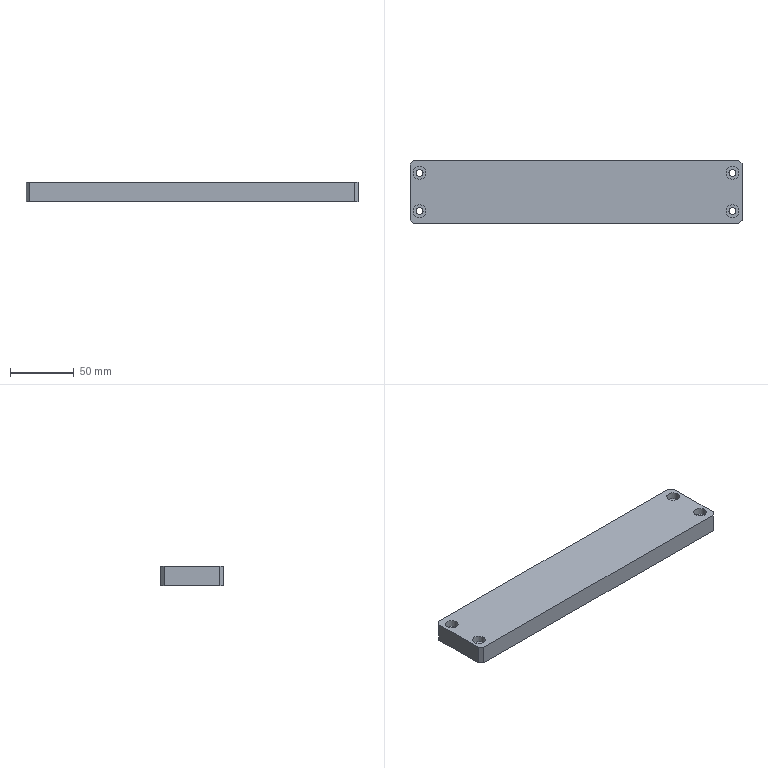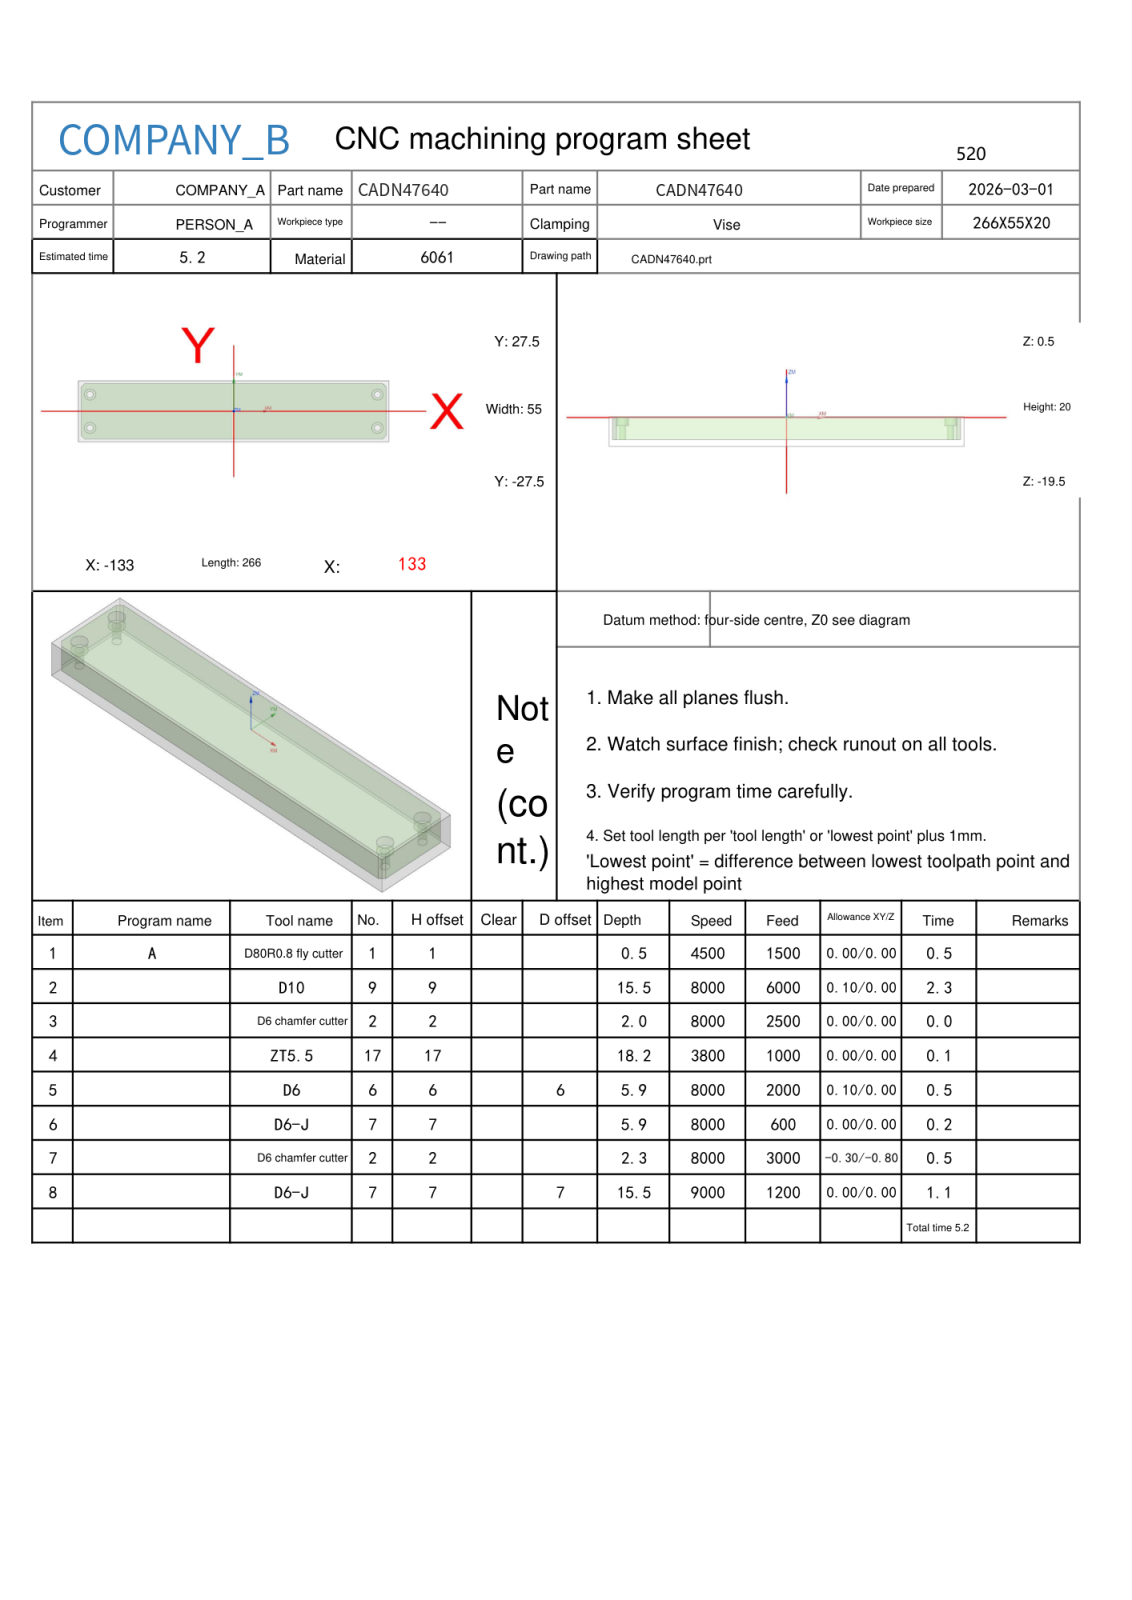NC program | NX | posted by the shop | part box 261 x 50 x 15 mm
Whole program:
%
O0001
(Machine time: 6.83 MIN)
(===Total Tool:6===)
(T1=D80R0.8 fly cutter D=80.  R=0.8  D-  H01 Z=0.    )
(T9=D10     D=10.  R=0.   D-  H09 Z=-15.  )
(T2=D6 chamfer cutter   D=6.   R=0.   D-  H02 Z=-1.8  )
(T17=ZT5.5  D=5.5  DR_a=118 D-  H17 Z=-17.65)
(T6=D6      D=6.   R=0.   D6  H06 Z=-5.4  )
(T7=D6-J    D=6.   R=0.   D-  H07 Z=-15.  )
G80 G90 G17 G49 G40
G91 G28 Z0
M01
N1 T01 M06
(D80R0.8 fly cutter D=80. R=0.8 H=01 ce=0.00 di=0.00)
G00 G90 G54 X-175.5 Y21.667 M03 S4500
G43 H01 Z50.
M08
Z2.
G01 Z0.0 F1500.
X-170.5
X170.5
Y-21.667
X-170.5
X-175.5
Z2.
G00 Z50.
G91 G28 Z0.0
M05
M09
G91 G28 Z0.0
M01
N2 T09 M06
(D10  D=10. R=0. H=09 ce=0.10 di=0.00)
G00 G90 G54 X0.0 Y-30.1 M03 S8000
G43 H09 Z50.
M08
Z.5
G01 X-127.5 Z.347 F6000.
G02 X-131.106 Y-28.606 Z.342 I0.0 J5.1
G01 X-134.106 Y-25.606 Z.337
G02 X-135.6 Y-22. Z.333 I3.606 J3.606
G01 Y22. Z.28
G02 X-134.106 Y25.606 Z.275 I5.1 J0.0
G01 X-131.106 Y28.606 Z.27
G02 X-127.5 Y30.1 Z.265 I3.606 J-3.606
G01 X127.5 Z-.04
G02 X131.106 Y28.606 Z-.045 I0.0 J-5.1
G01 X134.106 Y25.606 Z-.05
G02 X135.6 Y22. Z-.055 I-3.606 J-3.606
G01 Y-22. Z-.108
G02 X134.106 Y-25.606 Z-.112 I-5.1 J0.0
G01 X131.106 Y-28.606 Z-.117
G02 X127.5 Y-30.1 Z-.122 I-3.606 J3.606
G01 X-127.5 Z-.428
G02 X-131.106 Y-28.606 Z-.433 I0.0 J5.1
G01 X-134.106 Y-25.606 Z-.438
G02 X-135.6 Y-22. Z-.442 I3.606 J3.606
G01 Y22. Z-.495
G02 X-134.106 Y25.606 Z-.5 I5.1 J0.0
G01 X-131.106 Y28.606 Z-.505
G02 X-127.5 Y30.1 Z-.51 I3.606 J-3.606
G01 X127.5 Z-.815
G02 X131.106 Y28.606 Z-.82 I0.0 J-5.1
G01 X134.106 Y25.606 Z-.825
G02 X135.6 Y22. Z-.83 I-3.606 J-3.606
G01 Y-22. Z-.883
G02 X134.106 Y-25.606 Z-.887 I-5.1 J0.0
G01 X131.106 Y-28.606 Z-.892
G02 X127.5 Y-30.1 Z-.897 I-3.606 J3.606
G01 X-127.5 Z-1.203
G02 X-131.106 Y-28.606 Z-1.208 I0.0 J5.1
G01 X-134.106 Y-25.606 Z-1.213
G02 X-135.6 Y-22. Z-1.217 I3.606 J3.606
G01 Y22. Z-1.27
G02 X-134.106 Y25.606 Z-1.275 I5.1 J0.0
G01 X-131.106 Y28.606 Z-1.28
G02 X-127.5 Y30.1 Z-1.285 I3.606 J-3.606
G01 X127.5 Z-1.59
G02 X131.106 Y28.606 Z-1.595 I0.0 J-5.1
G01 X134.106 Y25.606 Z-1.6
G02 X135.6 Y22. Z-1.605 I-3.606 J-3.606
G01 Y-22. Z-1.658
G02 X134.106 Y-25.606 Z-1.662 I-5.1 J0.0
G01 X131.106 Y-28.606 Z-1.667
G02 X127.5 Y-30.1 Z-1.672 I-3.606 J3.606
G01 X-127.5 Z-1.978
G02 X-131.106 Y-28.606 Z-1.983 I0.0 J5.1
G01 X-134.106 Y-25.606 Z-1.988
G02 X-135.6 Y-22. Z-1.992 I3.606 J3.606
G01 Y22. Z-2.045
G02 X-134.106 Y25.606 Z-2.05 I5.1 J0.0
G01 X-131.106 Y28.606 Z-2.055
G02 X-127.5 Y30.1 Z-2.06 I3.606 J-3.606
G01 X127.5 Z-2.365
G02 X131.106 Y28.606 Z-2.37 I0.0 J-5.1
G01 X134.106 Y25.606 Z-2.375
G02 X135.6 Y22. Z-2.38 I-3.606 J-3.606
G01 Y-22. Z-2.433
G02 X134.106 Y-25.606 Z-2.437 I-5.1 J0.0
G01 X131.106 Y-28.606 Z-2.442
G02 X127.5 Y-30.1 Z-2.447 I-3.606 J3.606
G01 X-127.5 Z-2.753
G02 X-131.106 Y-28.606 Z-2.758 I0.0 J5.1
G01 X-134.106 Y-25.606 Z-2.763
G02 X-135.6 Y-22. Z-2.767 I3.606 J3.606
G01 Y22. Z-2.82
G02 X-134.106 Y25.606 Z-2.825 I5.1 J0.0
G01 X-131.106 Y28.606 Z-2.83
G02 X-127.5 Y30.1 Z-2.835 I3.606 J-3.606
G01 X127.5 Z-3.14
G02 X131.106 Y28.606 Z-3.145 I0.0 J-5.1
G01 X134.106 Y25.606 Z-3.15
G02 X135.6 Y22. Z-3.155 I-3.606 J-3.606
G01 Y-22. Z-3.208
G02 X134.106 Y-25.606 Z-3.212 I-5.1 J0.0
G01 X131.106 Y-28.606 Z-3.217
G02 X127.5 Y-30.1 Z-3.222 I-3.606 J3.606
G01 X-127.5 Z-3.528
G02 X-131.106 Y-28.606 Z-3.533 I0.0 J5.1
G01 X-134.106 Y-25.606 Z-3.538
G02 X-135.6 Y-22. Z-3.542 I3.606 J3.606
G01 Y22. Z-3.595
G02 X-134.106 Y25.606 Z-3.6 I5.1 J0.0
G01 X-131.106 Y28.606 Z-3.605
G02 X-127.5 Y30.1 Z-3.61 I3.606 J-3.606
G01 X127.5 Z-3.915
G02 X131.106 Y28.606 Z-3.92 I0.0 J-5.1
G01 X134.106 Y25.606 Z-3.925
G02 X135.6 Y22. Z-3.93 I-3.606 J-3.606
G01 Y-22. Z-3.983
G02 X134.106 Y-25.606 Z-3.987 I-5.1 J0.0
G01 X131.106 Y-28.606 Z-3.992
G02 X127.5 Y-30.1 Z-3.997 I-3.606 J3.606
G01 X-127.5 Z-4.303
G02 X-131.106 Y-28.606 Z-4.308 I0.0 J5.1
G01 X-134.106 Y-25.606 Z-4.313
G02 X-135.6 Y-22. Z-4.317 I3.606 J3.606
G01 Y22. Z-4.37
G02 X-134.106 Y25.606 Z-4.375 I5.1 J0.0
G01 X-131.106 Y28.606 Z-4.38
G02 X-127.5 Y30.1 Z-4.385 I3.606 J-3.606
G01 X127.5 Z-4.69
G02 X131.106 Y28.606 Z-4.695 I0.0 J-5.1
G01 X134.106 Y25.606 Z-4.7
G02 X135.6 Y22. Z-4.705 I-3.606 J-3.606
G01 Y-22. Z-4.758
G02 X134.106 Y-25.606 Z-4.762 I-5.1 J0.0
G01 X131.106 Y-28.606 Z-4.767
G02 X127.5 Y-30.1 Z-4.772 I-3.606 J3.606
G01 X-127.5 Z-5.078
G02 X-131.106 Y-28.606 Z-5.083 I0.0 J5.1
G01 X-134.106 Y-25.606 Z-5.088
G02 X-135.6 Y-22. Z-5.092 I3.606 J3.606
G01 Y22. Z-5.145
G02 X-134.106 Y25.606 Z-5.15 I5.1 J0.0
G01 X-131.106 Y28.606 Z-5.155
G02 X-127.5 Y30.1 Z-5.16 I3.606 J-3.606
G01 X127.5 Z-5.465
G02 X131.106 Y28.606 Z-5.47 I0.0 J-5.1
G01 X134.106 Y25.606 Z-5.475
G02 X135.6 Y22. Z-5.48 I-3.606 J-3.606
G01 Y-22. Z-5.533
G02 X134.106 Y-25.606 Z-5.537 I-5.1 J0.0
G01 X131.106 Y-28.606 Z-5.542
G02 X127.5 Y-30.1 Z-5.547 I-3.606 J3.606
G01 X-127.5 Z-5.853
G02 X-131.106 Y-28.606 Z-5.858 I0.0 J5.1
G01 X-134.106 Y-25.606 Z-5.863
G02 X-135.6 Y-22. Z-5.867 I3.606 J3.606
G01 Y22. Z-5.92
G02 X-134.106 Y25.606 Z-5.925 I5.1 J0.0
G01 X-131.106 Y28.606 Z-5.93
G02 X-127.5 Y30.1 Z-5.935 I3.606 J-3.606
G01 X127.5 Z-6.24
G02 X131.106 Y28.606 Z-6.245 I0.0 J-5.1
G01 X134.106 Y25.606 Z-6.25
G02 X135.6 Y22. Z-6.255 I-3.606 J-3.606
G01 Y-22. Z-6.308
G02 X134.106 Y-25.606 Z-6.312 I-5.1 J0.0
G01 X131.106 Y-28.606 Z-6.317
G02 X127.5 Y-30.1 Z-6.322 I-3.606 J3.606
G01 X-127.5 Z-6.628
G02 X-131.106 Y-28.606 Z-6.633 I0.0 J5.1
G01 X-134.106 Y-25.606 Z-6.638
G02 X-135.6 Y-22. Z-6.642 I3.606 J3.606
G01 Y22. Z-6.695
G02 X-134.106 Y25.606 Z-6.7 I5.1 J0.0
G01 X-131.106 Y28.606 Z-6.705
G02 X-127.5 Y30.1 Z-6.71 I3.606 J-3.606
G01 X127.5 Z-7.015
G02 X131.106 Y28.606 Z-7.02 I0.0 J-5.1
G01 X134.106 Y25.606 Z-7.025
G02 X135.6 Y22. Z-7.03 I-3.606 J-3.606
G01 Y-22. Z-7.083
G02 X134.106 Y-25.606 Z-7.087 I-5.1 J0.0
G01 X131.106 Y-28.606 Z-7.092
G02 X127.5 Y-30.1 Z-7.097 I-3.606 J3.606
G01 X-127.5 Z-7.403
G02 X-131.106 Y-28.606 Z-7.408 I0.0 J5.1
G01 X-134.106 Y-25.606 Z-7.413
G02 X-135.6 Y-22. Z-7.417 I3.606 J3.606
G01 Y22. Z-7.47
G02 X-134.106 Y25.606 Z-7.475 I5.1 J0.0
G01 X-131.106 Y28.606 Z-7.48
G02 X-127.5 Y30.1 Z-7.485 I3.606 J-3.606
G01 X127.5 Z-7.79
G02 X131.106 Y28.606 Z-7.795 I0.0 J-5.1
G01 X134.106 Y25.606 Z-7.8
G02 X135.6 Y22. Z-7.805 I-3.606 J-3.606
G01 Y-22. Z-7.858
G02 X134.106 Y-25.606 Z-7.862 I-5.1 J0.0
G01 X131.106 Y-28.606 Z-7.867
G02 X127.5 Y-30.1 Z-7.872 I-3.606 J3.606
G01 X-127.5 Z-8.178
G02 X-131.106 Y-28.606 Z-8.183 I0.0 J5.1
G01 X-134.106 Y-25.606 Z-8.188
G02 X-135.6 Y-22. Z-8.192 I3.606 J3.606
G01 Y22. Z-8.245
G02 X-134.106 Y25.606 Z-8.25 I5.1 J0.0
G01 X-131.106 Y28.606 Z-8.255
G02 X-127.5 Y30.1 Z-8.26 I3.606 J-3.606
G01 X127.5 Z-8.565
G02 X131.106 Y28.606 Z-8.57 I0.0 J-5.1
G01 X134.106 Y25.606 Z-8.575
G02 X135.6 Y22. Z-8.58 I-3.606 J-3.606
G01 Y-22. Z-8.633
G02 X134.106 Y-25.606 Z-8.637 I-5.1 J0.0
G01 X131.106 Y-28.606 Z-8.642
G02 X127.5 Y-30.1 Z-8.647 I-3.606 J3.606
G01 X-127.5 Z-8.953
G02 X-131.106 Y-28.606 Z-8.958 I0.0 J5.1
G01 X-134.106 Y-25.606 Z-8.963
G02 X-135.6 Y-22. Z-8.967 I3.606 J3.606
G01 Y22. Z-9.02
G02 X-134.106 Y25.606 Z-9.025 I5.1 J0.0
G01 X-131.106 Y28.606 Z-9.03
G02 X-127.5 Y30.1 Z-9.035 I3.606 J-3.606
G01 X127.5 Z-9.34
G02 X131.106 Y28.606 Z-9.345 I0.0 J-5.1
G01 X134.106 Y25.606 Z-9.35
G02 X135.6 Y22. Z-9.355 I-3.606 J-3.606
G01 Y-22. Z-9.408
G02 X134.106 Y-25.606 Z-9.412 I-5.1 J0.0
G01 X131.106 Y-28.606 Z-9.417
G02 X127.5 Y-30.1 Z-9.422 I-3.606 J3.606
G01 X-127.5 Z-9.728
G02 X-131.106 Y-28.606 Z-9.733 I0.0 J5.1
G01 X-134.106 Y-25.606 Z-9.738
G02 X-135.6 Y-22. Z-9.742 I3.606 J3.606
G01 Y22. Z-9.795
G02 X-134.106 Y25.606 Z-9.8 I5.1 J0.0
G01 X-131.106 Y28.606 Z-9.805
G02 X-127.5 Y30.1 Z-9.81 I3.606 J-3.606
G01 X127.5 Z-10.115
G02 X131.106 Y28.606 Z-10.12 I0.0 J-5.1
G01 X134.106 Y25.606 Z-10.125
G02 X135.6 Y22. Z-10.13 I-3.606 J-3.606
G01 Y-22. Z-10.183
G02 X134.106 Y-25.606 Z-10.187 I-5.1 J0.0
G01 X131.106 Y-28.606 Z-10.192
G02 X127.5 Y-30.1 Z-10.197 I-3.606 J3.606
G01 X-127.5 Z-10.503
G02 X-131.106 Y-28.606 Z-10.508 I0.0 J5.1
G01 X-134.106 Y-25.606 Z-10.513
G02 X-135.6 Y-22. Z-10.517 I3.606 J3.606
G01 Y22. Z-10.57
G02 X-134.106 Y25.606 Z-10.575 I5.1 J0.0
G01 X-131.106 Y28.606 Z-10.58
G02 X-127.5 Y30.1 Z-10.585 I3.606 J-3.606
G01 X127.5 Z-10.89
G02 X131.106 Y28.606 Z-10.895 I0.0 J-5.1
G01 X134.106 Y25.606 Z-10.9
G02 X135.6 Y22. Z-10.905 I-3.606 J-3.606
G01 Y-22. Z-10.958
G02 X134.106 Y-25.606 Z-10.962 I-5.1 J0.0
G01 X131.106 Y-28.606 Z-10.967
G02 X127.5 Y-30.1 Z-10.972 I-3.606 J3.606
G01 X-127.5 Z-11.278
G02 X-131.106 Y-28.606 Z-11.283 I0.0 J5.1
G01 X-134.106 Y-25.606 Z-11.288
G02 X-135.6 Y-22. Z-11.292 I3.606 J3.606
G01 Y22. Z-11.345
G02 X-134.106 Y25.606 Z-11.35 I5.1 J0.0
G01 X-131.106 Y28.606 Z-11.355
G02 X-127.5 Y30.1 Z-11.36 I3.606 J-3.606
G01 X127.5 Z-11.665
G02 X131.106 Y28.606 Z-11.67 I0.0 J-5.1
G01 X134.106 Y25.606 Z-11.675
G02 X135.6 Y22. Z-11.68 I-3.606 J-3.606
G01 Y-22. Z-11.733
G02 X134.106 Y-25.606 Z-11.737 I-5.1 J0.0
G01 X131.106 Y-28.606 Z-11.742
G02 X127.5 Y-30.1 Z-11.747 I-3.606 J3.606
G01 X-127.5 Z-12.053
G02 X-131.106 Y-28.606 Z-12.058 I0.0 J5.1
G01 X-134.106 Y-25.606 Z-12.063
G02 X-135.6 Y-22. Z-12.067 I3.606 J3.606
G01 Y22. Z-12.12
G02 X-134.106 Y25.606 Z-12.125 I5.1 J0.0
G01 X-131.106 Y28.606 Z-12.13
G02 X-127.5 Y30.1 Z-12.135 I3.606 J-3.606
G01 X127.5 Z-12.44
G02 X131.106 Y28.606 Z-12.445 I0.0 J-5.1
G01 X134.106 Y25.606 Z-12.45
G02 X135.6 Y22. Z-12.455 I-3.606 J-3.606
G01 Y-22. Z-12.508
G02 X134.106 Y-25.606 Z-12.512 I-5.1 J0.0
G01 X131.106 Y-28.606 Z-12.517
G02 X127.5 Y-30.1 Z-12.522 I-3.606 J3.606
G01 X-127.5 Z-12.828
G02 X-131.106 Y-28.606 Z-12.833 I0.0 J5.1
G01 X-134.106 Y-25.606 Z-12.838
G02 X-135.6 Y-22. Z-12.842 I3.606 J3.606
G01 Y22. Z-12.895
G02 X-134.106 Y25.606 Z-12.9 I5.1 J0.0
G01 X-131.106 Y28.606 Z-12.905
G02 X-127.5 Y30.1 Z-12.91 I3.606 J-3.606
G01 X127.5 Z-13.215
G02 X131.106 Y28.606 Z-13.22 I0.0 J-5.1
G01 X134.106 Y25.606 Z-13.225
G02 X135.6 Y22. Z-13.23 I-3.606 J-3.606
G01 Y-22. Z-13.283
G02 X134.106 Y-25.606 Z-13.287 I-5.1 J0.0
G01 X131.106 Y-28.606 Z-13.292
G02 X127.5 Y-30.1 Z-13.297 I-3.606 J3.606
G01 X-127.5 Z-13.603
G02 X-131.106 Y-28.606 Z-13.608 I0.0 J5.1
G01 X-134.106 Y-25.606 Z-13.613
G02 X-135.6 Y-22. Z-13.617 I3.606 J3.606
G01 Y22. Z-13.67
G02 X-134.106 Y25.606 Z-13.675 I5.1 J0.0
G01 X-131.106 Y28.606 Z-13.68
G02 X-127.5 Y30.1 Z-13.685 I3.606 J-3.606
G01 X127.5 Z-13.99
G02 X131.106 Y28.606 Z-13.995 I0.0 J-5.1
G01 X134.106 Y25.606 Z-14.
G02 X135.6 Y22. Z-14.005 I-3.606 J-3.606
G01 Y-22. Z-14.058
G02 X134.106 Y-25.606 Z-14.062 I-5.1 J0.0
G01 X131.106 Y-28.606 Z-14.067
G02 X127.5 Y-30.1 Z-14.072 I-3.606 J3.606
G01 X-127.5 Z-14.378
G02 X-131.106 Y-28.606 Z-14.383 I0.0 J5.1
G01 X-134.106 Y-25.606 Z-14.388
G02 X-135.6 Y-22. Z-14.392 I3.606 J3.606
G01 Y22. Z-14.445
G02 X-134.106 Y25.606 Z-14.45 I5.1 J0.0
G01 X-131.106 Y28.606 Z-14.455
G02 X-127.5 Y30.1 Z-14.46 I3.606 J-3.606
G01 X127.5 Z-14.765
G02 X131.106 Y28.606 Z-14.77 I0.0 J-5.1
G01 X134.106 Y25.606 Z-14.775
G02 X135.6 Y22. Z-14.78 I-3.606 J-3.606
G01 Y-22. Z-14.833
G02 X134.106 Y-25.606 Z-14.837 I-5.1 J0.0
G01 X131.106 Y-28.606 Z-14.842
G02 X127.5 Y-30.1 Z-14.847 I-3.606 J3.606
G01 X0.0 Z-15.
X-127.5
G02 X-131.106 Y-28.606 I0.0 J5.1
G01 X-134.106 Y-25.606
G02 X-135.6 Y-22. I3.606 J3.606
G01 Y22.
G02 X-134.106 Y25.606 I5.1 J0.0
G01 X-131.106 Y28.606
G02 X-127.5 Y30.1 I3.606 J-3.606
G01 X127.5
G02 X131.106 Y28.606 I0.0 J-5.1
G01 X134.106 Y25.606
G02 X135.6 Y22. I-3.606 J-3.606
G01 Y-22.
G02 X134.106 Y-25.606 I-5.1 J0.0
G01 X131.106 Y-28.606
G02 X127.5 Y-30.1 I-3.606 J3.606
G01 X0.0
X-.5
Z-14.
G00 Z50.
G91 G28 Z0.0
M05
M09
G91 G28 Z0.0
M01
N3 T02 M06
(D6 chamfer cutter D=6. R=0. H=02 ce=0.00 di=0.00)
G00 G90 G54 X-123. Y-15. M03 S8000
G43 H02 Z50.
M08
G98 G81 X-123. Y-15. Z-1.5 R1. F2500.
Y15.
X123.
Y-15.
G80
G00 Z50.
G91 G28 Z0.0
M05
M09
G91 G28 Z0.0
M01
N4 T17 M06
(ZT5.5 D=5.5 DR_a=118 H=17)
G00 G90 G54 X-123. Y-15. M03 S3800
G43 H17 Z50.
M08
G98 G83 X-123. Y-15. Z-17.652 R1. F1000. Q3.
Y15.
X123.
Y-15.
G80
G00 Z50.
G91 G28 Z0.0
M05
M09
G91 G28 Z0.0
M01
N5 T06 M06
(D6  D=6. R=0. H=06 ce=0.10 di=0.00)
G00 G90 G54 X-123. Y-15. M03 S8000
G43 H06 Z50.
M08
Z.3
G41 D06
G01 X-123.007 Y-15.1 F2000.
G03 X-122.056 Y-15.956 I.951 J.1
X-121.1 Y-15. I0.0 J.956
X-121.1 Y-15. Z-.05 I-1.9 J0.0
X-121.1 Y-15. Z-.4 I-1.9 J0.0
X-121.1 Y-15. Z-.75 I-1.9 J0.0
X-121.1 Y-15. Z-1.1 I-1.9 J0.0
X-121.1 Y-15. Z-1.45 I-1.9 J0.0
X-121.1 Y-15. Z-1.8 I-1.9 J0.0
X-121.1 Y-15. Z-2.15 I-1.9 J0.0
X-121.1 Y-15. Z-2.5 I-1.9 J0.0
X-121.1 Y-15. Z-2.85 I-1.9 J0.0
X-121.1 Y-15. Z-3.2 I-1.9 J0.0
X-121.1 Y-15. Z-3.55 I-1.9 J0.0
X-121.1 Y-15. Z-3.9 I-1.9 J0.0
X-121.1 Y-15. Z-4.25 I-1.9 J0.0
X-121.1 Y-15. Z-4.6 I-1.9 J0.0
X-121.1 Y-15. Z-4.95 I-1.9 J0.0
X-121.1 Y-15. Z-5.3 I-1.9 J0.0
X-123.423 Y-13.148 Z-5.4 I-1.9 J0.0
X-124.9 Y-15. I.423 J-1.852
X-123. Y-16.9 I1.9 J0.0
X-121.1 Y-15. I0.0 J1.9
X-123. Y-13.1 I-1.9 J0.0
X-123.423 Y-13.148 I0.0 J-1.9
X-124.166 Y-14.08 I.213 J-.932
X-123.21 Y-15.036 I.956 J0.0
G01 X-123.096 Y-15.029
G40 X-123. Y-15.
G00 Z50.
Y15.
Z.3
G41 D06
G01 X-123.007 Y14.9
G03 X-122.056 Y14.044 I.951 J.1
X-121.1 Y15. I0.0 J.956
X-121.1 Y15. Z-.05 I-1.9 J0.0
X-121.1 Y15. Z-.4 I-1.9 J0.0
X-121.1 Y15. Z-.75 I-1.9 J0.0
X-121.1 Y15. Z-1.1 I-1.9 J0.0
X-121.1 Y15. Z-1.45 I-1.9 J0.0
X-121.1 Y15. Z-1.8 I-1.9 J0.0
X-121.1 Y15. Z-2.15 I-1.9 J0.0
X-121.1 Y15. Z-2.5 I-1.9 J0.0
X-121.1 Y15. Z-2.85 I-1.9 J0.0
X-121.1 Y15. Z-3.2 I-1.9 J0.0
X-121.1 Y15. Z-3.55 I-1.9 J0.0
X-121.1 Y15. Z-3.9 I-1.9 J0.0
X-121.1 Y15. Z-4.25 I-1.9 J0.0
X-121.1 Y15. Z-4.6 I-1.9 J0.0
X-121.1 Y15. Z-4.95 I-1.9 J0.0
X-121.1 Y15. Z-5.3 I-1.9 J0.0
X-123.423 Y16.852 Z-5.4 I-1.9 J0.0
X-124.9 Y15. I.423 J-1.852
X-123. Y13.1 I1.9 J0.0
X-121.1 Y15. I0.0 J1.9
X-123. Y16.9 I-1.9 J0.0
X-123.423 Y16.852 I0.0 J-1.9
X-124.166 Y15.92 I.213 J-.932
X-123.21 Y14.964 I.956 J0.0
G01 X-123.096 Y14.971
G40 X-123. Y15.
G00 Z50.
X123.
Z.3
G41 D06
G01 X122.993 Y14.9
G03 X123.944 Y14.044 I.951 J.1
X124.9 Y15. I0.0 J.956
X124.9 Y15. Z-.05 I-1.9 J0.0
X124.9 Y15. Z-.4 I-1.9 J0.0
X124.9 Y15. Z-.75 I-1.9 J0.0
X124.9 Y15. Z-1.1 I-1.9 J0.0
X124.9 Y15. Z-1.45 I-1.9 J0.0
X124.9 Y15. Z-1.8 I-1.9 J0.0
X124.9 Y15. Z-2.15 I-1.9 J0.0
X124.9 Y15. Z-2.5 I-1.9 J0.0
X124.9 Y15. Z-2.85 I-1.9 J0.0
X124.9 Y15. Z-3.2 I-1.9 J0.0
X124.9 Y15. Z-3.55 I-1.9 J0.0
X124.9 Y15. Z-3.9 I-1.9 J0.0
X124.9 Y15. Z-4.25 I-1.9 J0.0
X124.9 Y15. Z-4.6 I-1.9 J0.0
X124.9 Y15. Z-4.95 I-1.9 J0.0
X124.9 Y15. Z-5.3 I-1.9 J0.0
X122.577 Y16.852 Z-5.4 I-1.9 J0.0
X121.1 Y15. I.423 J-1.852
X123. Y13.1 I1.9 J0.0
X124.9 Y15. I0.0 J1.9
X123. Y16.9 I-1.9 J0.0
X122.577 Y16.852 I0.0 J-1.9
X121.834 Y15.92 I.213 J-.932
X122.79 Y14.964 I.956 J0.0
G01 X122.904 Y14.971
G40 X123. Y15.
G00 Z50.
Y-15.
Z.3
G41 D06
G01 X122.993 Y-15.1
G03 X123.944 Y-15.956 I.951 J.1
X124.9 Y-15. I0.0 J.956
X124.9 Y-15. Z-.05 I-1.9 J0.0
X124.9 Y-15. Z-.4 I-1.9 J0.0
X124.9 Y-15. Z-.75 I-1.9 J0.0
X124.9 Y-15. Z-1.1 I-1.9 J0.0
X124.9 Y-15. Z-1.45 I-1.9 J0.0
X124.9 Y-15. Z-1.8 I-1.9 J0.0
X124.9 Y-15. Z-2.15 I-1.9 J0.0
X124.9 Y-15. Z-2.5 I-1.9 J0.0
X124.9 Y-15. Z-2.85 I-1.9 J0.0
X124.9 Y-15. Z-3.2 I-1.9 J0.0
X124.9 Y-15. Z-3.55 I-1.9 J0.0
X124.9 Y-15. Z-3.9 I-1.9 J0.0
X124.9 Y-15. Z-4.25 I-1.9 J0.0
X124.9 Y-15. Z-4.6 I-1.9 J0.0
X124.9 Y-15. Z-4.95 I-1.9 J0.0
X124.9 Y-15. Z-5.3 I-1.9 J0.0
X122.577 Y-13.148 Z-5.4 I-1.9 J0.0
X121.1 Y-15. I.423 J-1.852
X123. Y-16.9 I1.9 J0.0
X124.9 Y-15. I0.0 J1.9
X123. Y-13.1 I-1.9 J0.0
X122.577 Y-13.148 I0.0 J-1.9
X121.834 Y-14.08 I.213 J-.932
X122.79 Y-15.036 I.956 J0.0
G01 X122.904 Y-15.029
G40 X123. Y-15.
G00 Z50.
G91 G28 Z0.0
M05
M09
G91 G28 Z0.0
M01
N6 T07 M06
(D6-J  D=6. R=0. H=07 ce=0.00 di=0.00)
G00 G90 G54 X-123. Y-15. M03 S8000
G43 H07 Z50.
M08
Z-5.4
G01 X-121.439 Y-15.351 F600.
X-121.36 Y-15.36
G03 X-121. Y-15. I0.0 J.36
X-123. Y-13. I-2. J0.0
X-125. Y-15. I0.0 J-2.
X-123. Y-17. I2. J0.0
X-121. Y-15. I0.0 J2.
X-121.062 Y-14.505 I-2. J0.0
X-121.411 Y-14.234 I-.349 J-.089
G01 X-121.574 Y-14.274
X-123. Y-15.
G00 Z50.
Y15.
Z-5.4
G01 X-121.439 Y14.649
X-121.36 Y14.64
G03 X-121. Y15. I0.0 J.36
X-123. Y17. I-2. J0.0
X-125. Y15. I0.0 J-2.
X-123. Y13. I2. J0.0
X-121. Y15. I0.0 J2.
X-121.062 Y15.495 I-2. J0.0
X-121.411 Y15.766 I-.349 J-.089
G01 X-121.574 Y15.726
X-123. Y15.
G00 Z50.
X123.
Z-5.4
G01 X124.561 Y14.649
X124.64 Y14.64
G03 X125. Y15. I0.0 J.36
X123. Y17. I-2. J0.0
X121. Y15. I0.0 J-2.
X123. Y13. I2. J0.0
X125. Y15. I0.0 J2.
X124.938 Y15.495 I-2. J0.0
X124.589 Y15.766 I-.349 J-.089
G01 X124.426 Y15.726
X123. Y15.
G00 Z50.
Y-15.
Z-5.4
G01 X124.561 Y-15.351
X124.64 Y-15.36
G03 X125. Y-15. I0.0 J.36
X123. Y-13. I-2. J0.0
X121. Y-15. I0.0 J-2.
X123. Y-17. I2. J0.0
X125. Y-15. I0.0 J2.
X124.938 Y-14.505 I-2. J0.0
X124.589 Y-14.234 I-.349 J-.089
G01 X124.426 Y-14.274
X123. Y-15.
G00 Z50.
G91 G28 Z0.0
M05
M09
G91 G28 Z0.0
M01
N7 T02 M06
(D6 chamfer cutter D=6. R=0. H=02 ce=0.00 di=0.00)
G00 G90 G54 X.25 Y-27.128 M03 S8000
G43 H02 Z50.
M08
Z2.099
G01 Z-1.5 F3000.
G03 X.33 Y-26.828 I-.52 J.3
X.03 Y-26.308 I-.6 J0.0
G01 X0.0 Y-26.3
X-127.5
X-127.754 Y-26.275
X-127.997 Y-26.201
X-128.222 Y-26.081
X-128.419 Y-25.919
X-131.419 Y-22.919
X-131.581 Y-22.722
X-131.701 Y-22.497
X-131.775 Y-22.254
X-131.8 Y-22.
Y22.
X-131.775 Y22.254
X-131.701 Y22.497
X-131.581 Y22.722
X-131.419 Y22.919
X-128.419 Y25.919
X-128.222 Y26.081
X-127.997 Y26.201
X-127.754 Y26.275
X-127.5 Y26.3
X127.5
X127.754 Y26.275
X127.997 Y26.201
X128.222 Y26.081
X128.419 Y25.919
X131.419 Y22.919
X131.581 Y22.722
X131.701 Y22.497
X131.775 Y22.254
X131.8 Y22.
Y-22.
X131.775 Y-22.254
X131.701 Y-22.497
X131.581 Y-22.722
X131.419 Y-22.919
X128.419 Y-25.919
X128.222 Y-26.081
X127.997 Y-26.201
X127.754 Y-26.275
X127.5 Y-26.3
X0.0
X-.03 Y-26.308
G03 X-.33 Y-26.828 I.3 J-.52
X-.25 Y-27.128 I.6 J0.0
G01 Z2.099
G00 Z50.
G00 G90 X-123.411 Y-12.534 M03 S8000
Z50.
Z-1.3
G01 Z-1.8 F600.
X-123.5 Y-12.
G03 X-126.5 Y-15. I0.0 J-3.
X-123. Y-18.5 I3.5 J0.0
X-119.5 Y-15. I0.0 J3.5
X-123. Y-11.5 I-3.5 J0.0
X-126.5 Y-15. I0.0 J-3.5
X-123.5 Y-18. I3. J0.0
G01 X-123.411 Y-17.466
Z-1.3
G00 Z50.
Y17.466
Z-1.3
G01 Z-1.8
X-123.5 Y18.
G03 X-126.5 Y15. I0.0 J-3.
X-123. Y11.5 I3.5 J0.0
X-119.5 Y15. I0.0 J3.5
X-123. Y18.5 I-3.5 J0.0
X-126.5 Y15. I0.0 J-3.5
X-123.5 Y12. I3. J0.0
G01 X-123.411 Y12.534
Z-1.3
G00 Z50.
X122.589 Y17.466
Z-1.3
G01 Z-1.8
X122.5 Y18.
G03 X119.5 Y15. I0.0 J-3.
X123. Y11.5 I3.5 J0.0
X126.5 Y15. I0.0 J3.5
X123. Y18.5 I-3.5 J0.0
X119.5 Y15. I0.0 J-3.5
X122.5 Y12. I3. J0.0
G01 X122.589 Y12.534
Z-1.3
G00 Z50.
Y-12.534
Z-1.3
G01 Z-1.8
X122.5 Y-12.
G03 X119.5 Y-15. I0.0 J-3.
X123. Y-18.5 I3.5 J0.0
X126.5 Y-15. I0.0 J3.5
X123. Y-11.5 I-3.5 J0.0
X119.5 Y-15. I0.0 J-3.5
X122.5 Y-18. I3. J0.0
G01 X122.589 Y-17.466
Z-1.3
G00 Z50.
G91 G28 Z0.0
M05
M09
G91 G28 Z0.0
M01
N8 T07 M06
(D6-J  D=6. R=0. H=07 ce=0.00 di=0.00)
G00 G90 G54 X-128.517 Y29.073 M03 S9000
G43 H07 Z50.
M08
Z-7.
G01 Z-7.5 F1200.
G41 D07
X-128.492 Y28.875
G03 X-127.5 Y28. I.992 J.125
G01 X127.5
G02 X129.621 Y27.121 I0.0 J-3.
G01 X132.621 Y24.121
G02 X133.5 Y22. I-2.121 J-2.121
G01 Y-22.
G02 X132.621 Y-24.121 I-3. J0.0
G01 X129.621 Y-27.121
G02 X127.5 Y-28. I-2.121 J2.121
G01 X-127.5
G02 X-129.621 Y-27.121 I0.0 J3.
G01 X-132.621 Y-24.121
G02 X-133.5 Y-22. I2.121 J2.121
G01 Y22.
G02 X-132.621 Y24.121 I3. J0.0
G01 X-129.621 Y27.121
G02 X-127.5 Y28. I2.121 J-2.121
G01 X-127.
G03 X-126. Y29. I0.0 J1.
G01 G40 Y29.2
Z-7.
G00 Z50.
X-128.517 Y29.073
Z-14.5
G01 Z-15.
G41 D07
X-128.492 Y28.875
G03 X-127.5 Y28. I.992 J.125
G01 X127.5
G02 X129.621 Y27.121 I0.0 J-3.
G01 X132.621 Y24.121
G02 X133.5 Y22. I-2.121 J-2.121
G01 Y-22.
G02 X132.621 Y-24.121 I-3. J0.0
G01 X129.621 Y-27.121
G02 X127.5 Y-28. I-2.121 J2.121
G01 X-127.5
G02 X-129.621 Y-27.121 I0.0 J3.
G01 X-132.621 Y-24.121
G02 X-133.5 Y-22. I2.121 J2.121
G01 Y22.
G02 X-132.621 Y24.121 I3. J0.0
G01 X-129.621 Y27.121
G02 X-127.5 Y28. I2.121 J-2.121
G01 X-127.
G03 X-126. Y29. I0.0 J1.
G01 G40 Y29.2
Z-14.5
G00 Z50.
M05
M09
G91 G28 Z0.0
G91 G28 Y0.0
M30
%